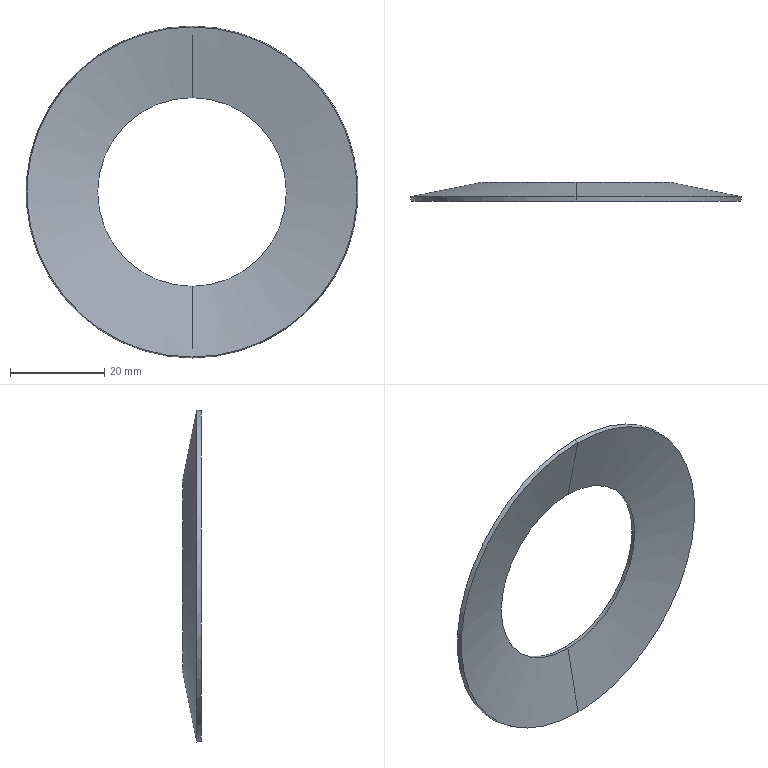Part | STEP file | disc spring2 | 1 solid | 8 faces | box 70.392 x 3.981 x 70.392 mm | volume 2653 mm3 | cone 8
STEP:
#1=CARTESIAN_POINT('',(0.,3.,-20.));
#2=VERTEX_POINT('',#1);
#3=CARTESIAN_POINT('',(0.,3.,20.));
#4=VERTEX_POINT('',#3);
#5=CARTESIAN_POINT('',(0.,3.,0.));
#6=DIRECTION('',(0.,1.,0.));
#7=DIRECTION('',(0.,0.,1.));
#8=AXIS2_PLACEMENT_3D('',#5,#6,#7);
#9=CIRCLE('',#8,20.);
#10=EDGE_CURVE('',#2,#4,#9,.T.);
#11=ORIENTED_EDGE('',*,*,#10,.T.);
#12=CARTESIAN_POINT('',(0.,0.,35.));
#13=VERTEX_POINT('',#12);
#14=CARTESIAN_POINT('',(0.,0.,35.));
#15=DIRECTION('',(0.,-0.1961,0.9806));
#16=VECTOR('',#15,1000.);
#17=LINE('',#14,#16);
#18=EDGE_CURVE('',#4,#13,#17,.T.);
#19=ORIENTED_EDGE('',*,*,#18,.T.);
#20=CARTESIAN_POINT('',(0.,0.,-35.));
#21=VERTEX_POINT('',#20);
#22=CARTESIAN_POINT('',(0.,0.,0.));
#23=DIRECTION('',(0.,1.,0.));
#24=DIRECTION('',(0.,0.,1.));
#25=AXIS2_PLACEMENT_3D('',#22,#23,#24);
#26=CIRCLE('',#25,35.);
#27=EDGE_CURVE('',#21,#13,#26,.T.);
#28=ORIENTED_EDGE('',*,*,#27,.F.);
#29=CARTESIAN_POINT('',(0.,0.,-35.));
#30=DIRECTION('',(0.,-0.1961,-0.9806));
#31=VECTOR('',#30,1000.);
#32=LINE('',#29,#31);
#33=EDGE_CURVE('',#2,#21,#32,.T.);
#34=ORIENTED_EDGE('',*,*,#33,.F.);
#35=EDGE_LOOP('',(#11,#19,#28,#34));
#36=FACE_OUTER_BOUND('',#35,.T.);
#37=CARTESIAN_POINT('',(0.,0.,0.));
#38=DIRECTION('',(0.,-1.,0.));
#39=DIRECTION('',(0.,0.,-1.));
#40=AXIS2_PLACEMENT_3D('',#37,#38,#39);
#41=CONICAL_SURFACE('',#40,35.,1.373);
#42=ADVANCED_FACE('',(#36),#41,.F.);
#43=ORIENTED_EDGE('',*,*,#10,.F.);
#44=CARTESIAN_POINT('',(0.,3.981,-20.196));
#45=VERTEX_POINT('',#44);
#46=CARTESIAN_POINT('',(0.,3.,-20.));
#47=DIRECTION('',(0.,0.9806,-0.1961));
#48=VECTOR('',#47,1000.);
#49=LINE('',#46,#48);
#50=EDGE_CURVE('',#2,#45,#49,.T.);
#51=ORIENTED_EDGE('',*,*,#50,.T.);
#52=CARTESIAN_POINT('',(0.,3.981,20.196));
#53=VERTEX_POINT('',#52);
#54=CARTESIAN_POINT('',(0.,3.981,0.));
#55=DIRECTION('',(0.,1.,0.));
#56=DIRECTION('',(0.,0.,1.));
#57=AXIS2_PLACEMENT_3D('',#54,#55,#56);
#58=CIRCLE('',#57,20.196);
#59=EDGE_CURVE('',#45,#53,#58,.T.);
#60=ORIENTED_EDGE('',*,*,#59,.T.);
#61=CARTESIAN_POINT('',(0.,3.,20.));
#62=DIRECTION('',(0.,0.9806,0.1961));
#63=VECTOR('',#62,1000.);
#64=LINE('',#61,#63);
#65=EDGE_CURVE('',#4,#53,#64,.T.);
#66=ORIENTED_EDGE('',*,*,#65,.F.);
#67=EDGE_LOOP('',(#43,#51,#60,#66));
#68=FACE_OUTER_BOUND('',#67,.T.);
#69=CARTESIAN_POINT('',(0.,3.,0.));
#70=DIRECTION('',(0.,1.,0.));
#71=DIRECTION('',(0.,0.,1.));
#72=AXIS2_PLACEMENT_3D('',#69,#70,#71);
#73=CONICAL_SURFACE('',#72,20.,0.1974);
#74=ADVANCED_FACE('',(#68),#73,.F.);
#75=CARTESIAN_POINT('',(0.,3.981,0.));
#76=DIRECTION('',(0.,1.,0.));
#77=DIRECTION('',(0.,0.,1.));
#78=AXIS2_PLACEMENT_3D('',#75,#76,#77);
#79=CIRCLE('',#78,20.196);
#80=EDGE_CURVE('',#53,#45,#79,.T.);
#81=ORIENTED_EDGE('',*,*,#80,.F.);
#82=CARTESIAN_POINT('',(0.,0.9806,35.196));
#83=VERTEX_POINT('',#82);
#84=CARTESIAN_POINT('',(0.,3.981,20.196));
#85=DIRECTION('',(0.,-0.1961,0.9806));
#86=VECTOR('',#85,1000.);
#87=LINE('',#84,#86);
#88=EDGE_CURVE('',#53,#83,#87,.T.);
#89=ORIENTED_EDGE('',*,*,#88,.T.);
#90=CARTESIAN_POINT('',(0.,0.9806,-35.196));
#91=VERTEX_POINT('',#90);
#92=CARTESIAN_POINT('',(0.,0.9806,0.));
#93=DIRECTION('',(0.,1.,0.));
#94=DIRECTION('',(0.,0.,1.));
#95=AXIS2_PLACEMENT_3D('',#92,#93,#94);
#96=CIRCLE('',#95,35.196);
#97=EDGE_CURVE('',#83,#91,#96,.T.);
#98=ORIENTED_EDGE('',*,*,#97,.T.);
#99=CARTESIAN_POINT('',(0.,3.981,-20.196));
#100=DIRECTION('',(0.,-0.1961,-0.9806));
#101=VECTOR('',#100,1000.);
#102=LINE('',#99,#101);
#103=EDGE_CURVE('',#45,#91,#102,.T.);
#104=ORIENTED_EDGE('',*,*,#103,.F.);
#105=EDGE_LOOP('',(#81,#89,#98,#104));
#106=FACE_OUTER_BOUND('',#105,.T.);
#107=CARTESIAN_POINT('',(0.,3.981,0.));
#108=DIRECTION('',(0.,-1.,0.));
#109=DIRECTION('',(0.,0.,-1.));
#110=AXIS2_PLACEMENT_3D('',#107,#108,#109);
#111=CONICAL_SURFACE('',#110,20.196,1.373);
#112=ADVANCED_FACE('',(#106),#111,.T.);
#113=CARTESIAN_POINT('',(0.,0.,0.));
#114=DIRECTION('',(0.,1.,0.));
#115=DIRECTION('',(0.,0.,1.));
#116=AXIS2_PLACEMENT_3D('',#113,#114,#115);
#117=CIRCLE('',#116,35.);
#118=EDGE_CURVE('',#13,#21,#117,.T.);
#119=ORIENTED_EDGE('',*,*,#118,.T.);
#120=CARTESIAN_POINT('',(0.,0.9806,-35.196));
#121=DIRECTION('',(0.,0.9806,-0.1961));
#122=VECTOR('',#121,1000.);
#123=LINE('',#120,#122);
#124=EDGE_CURVE('',#21,#91,#123,.T.);
#125=ORIENTED_EDGE('',*,*,#124,.T.);
#126=ORIENTED_EDGE('',*,*,#97,.F.);
#127=CARTESIAN_POINT('',(0.,0.9806,35.196));
#128=DIRECTION('',(0.,0.9806,0.1961));
#129=VECTOR('',#128,1000.);
#130=LINE('',#127,#129);
#131=EDGE_CURVE('',#13,#83,#130,.T.);
#132=ORIENTED_EDGE('',*,*,#131,.F.);
#133=EDGE_LOOP('',(#119,#125,#126,#132));
#134=FACE_OUTER_BOUND('',#133,.T.);
#135=CARTESIAN_POINT('',(0.,0.9806,0.));
#136=DIRECTION('',(0.,1.,0.));
#137=DIRECTION('',(0.,0.,1.));
#138=AXIS2_PLACEMENT_3D('',#135,#136,#137);
#139=CONICAL_SURFACE('',#138,35.196,0.1974);
#140=ADVANCED_FACE('',(#134),#139,.T.);
#141=ORIENTED_EDGE('',*,*,#124,.F.);
#142=ORIENTED_EDGE('',*,*,#27,.T.);
#143=ORIENTED_EDGE('',*,*,#131,.T.);
#144=CARTESIAN_POINT('',(0.,0.9806,0.));
#145=DIRECTION('',(0.,1.,0.));
#146=DIRECTION('',(0.,0.,1.));
#147=AXIS2_PLACEMENT_3D('',#144,#145,#146);
#148=CIRCLE('',#147,35.196);
#149=EDGE_CURVE('',#91,#83,#148,.T.);
#150=ORIENTED_EDGE('',*,*,#149,.F.);
#151=EDGE_LOOP('',(#141,#142,#143,#150));
#152=FACE_OUTER_BOUND('',#151,.T.);
#153=CARTESIAN_POINT('',(0.,0.9806,0.));
#154=DIRECTION('',(0.,1.,0.));
#155=DIRECTION('',(0.,0.,1.));
#156=AXIS2_PLACEMENT_3D('',#153,#154,#155);
#157=CONICAL_SURFACE('',#156,35.196,0.1974);
#158=ADVANCED_FACE('',(#152),#157,.T.);
#159=ORIENTED_EDGE('',*,*,#88,.F.);
#160=ORIENTED_EDGE('',*,*,#59,.F.);
#161=ORIENTED_EDGE('',*,*,#103,.T.);
#162=ORIENTED_EDGE('',*,*,#149,.T.);
#163=EDGE_LOOP('',(#159,#160,#161,#162));
#164=FACE_OUTER_BOUND('',#163,.T.);
#165=CARTESIAN_POINT('',(0.,3.981,0.));
#166=DIRECTION('',(0.,-1.,0.));
#167=DIRECTION('',(0.,0.,-1.));
#168=AXIS2_PLACEMENT_3D('',#165,#166,#167);
#169=CONICAL_SURFACE('',#168,20.196,1.373);
#170=ADVANCED_FACE('',(#164),#169,.T.);
#171=ORIENTED_EDGE('',*,*,#50,.F.);
#172=CARTESIAN_POINT('',(0.,3.,0.));
#173=DIRECTION('',(0.,1.,0.));
#174=DIRECTION('',(0.,0.,1.));
#175=AXIS2_PLACEMENT_3D('',#172,#173,#174);
#176=CIRCLE('',#175,20.);
#177=EDGE_CURVE('',#4,#2,#176,.T.);
#178=ORIENTED_EDGE('',*,*,#177,.F.);
#179=ORIENTED_EDGE('',*,*,#65,.T.);
#180=ORIENTED_EDGE('',*,*,#80,.T.);
#181=EDGE_LOOP('',(#171,#178,#179,#180));
#182=FACE_OUTER_BOUND('',#181,.T.);
#183=CARTESIAN_POINT('',(0.,3.,0.));
#184=DIRECTION('',(0.,1.,0.));
#185=DIRECTION('',(0.,0.,1.));
#186=AXIS2_PLACEMENT_3D('',#183,#184,#185);
#187=CONICAL_SURFACE('',#186,20.,0.1974);
#188=ADVANCED_FACE('',(#182),#187,.F.);
#189=ORIENTED_EDGE('',*,*,#18,.F.);
#190=ORIENTED_EDGE('',*,*,#177,.T.);
#191=ORIENTED_EDGE('',*,*,#33,.T.);
#192=ORIENTED_EDGE('',*,*,#118,.F.);
#193=EDGE_LOOP('',(#189,#190,#191,#192));
#194=FACE_OUTER_BOUND('',#193,.T.);
#195=CARTESIAN_POINT('',(0.,0.,0.));
#196=DIRECTION('',(0.,-1.,0.));
#197=DIRECTION('',(0.,0.,-1.));
#198=AXIS2_PLACEMENT_3D('',#195,#196,#197);
#199=CONICAL_SURFACE('',#198,35.,1.373);
#200=ADVANCED_FACE('',(#194),#199,.F.);
#201=CLOSED_SHELL('',(#42,#74,#112,#140,#158,#170,#188,#200));
#202=MANIFOLD_SOLID_BREP('',#201);
#203=CARTESIAN_POINT('',(0.,0.,0.));
#204=DIRECTION('',(0.,0.,1.));
#205=DIRECTION('',(1.,0.,0.));
#206=AXIS2_PLACEMENT_3D('',#203,#204,#205);
#207=(LENGTH_UNIT()NAMED_UNIT(*)SI_UNIT(.MILLI.,.METRE.));
#208=UNCERTAINTY_MEASURE_WITH_UNIT(LENGTH_MEASURE(0.00001),#207,'','');
#209=(NAMED_UNIT(*)PLANE_ANGLE_UNIT()SI_UNIT($,.RADIAN.));
#210=(NAMED_UNIT(*)SI_UNIT($,.STERADIAN.)SOLID_ANGLE_UNIT());
#211=(GEOMETRIC_REPRESENTATION_CONTEXT(3)GLOBAL_UNCERTAINTY_ASSIGNED_CONTEXT((#208))GLOBAL_UNIT_ASSIGNED_CONTEXT((#207,#209,#210))REPRESENTATION_CONTEXT('',''));
#212=ADVANCED_BREP_SHAPE_REPRESENTATION('',(#202,#206),#211);